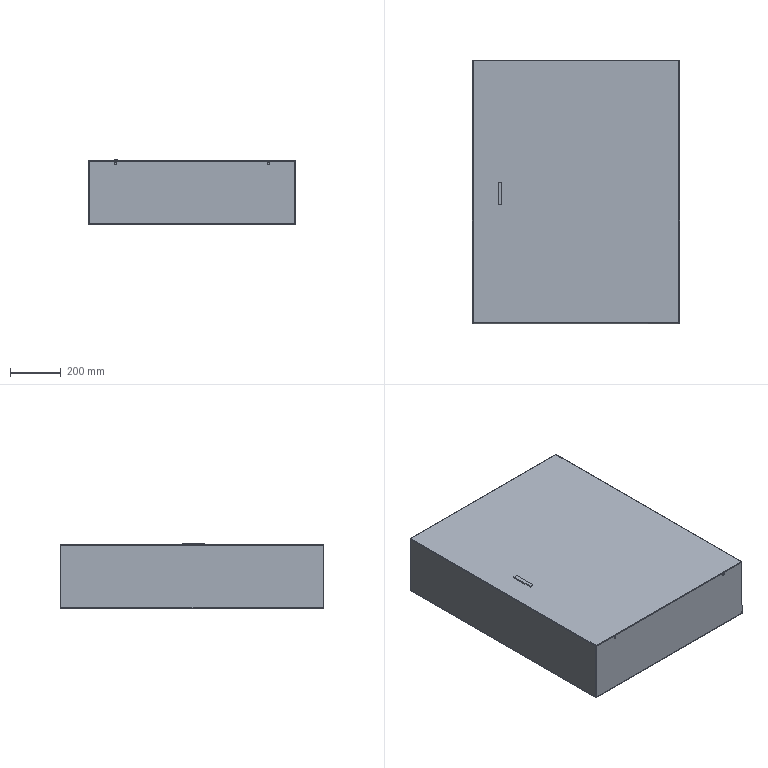Part | SolidWorks | features ICE 9, EdgeFlange 2, LPattern 2, Emboss 1, FlatPattern 1, SMBaseFlange 1, SheetMetal 1 | 1 solid | 79 faces | box 812 x 1034 x 255 mm | volume 2671023 mm3 | plane 43 | cylinder 20 | spline 16 | commonest cylinder face diameters 3 x8 6 x8 9 x4